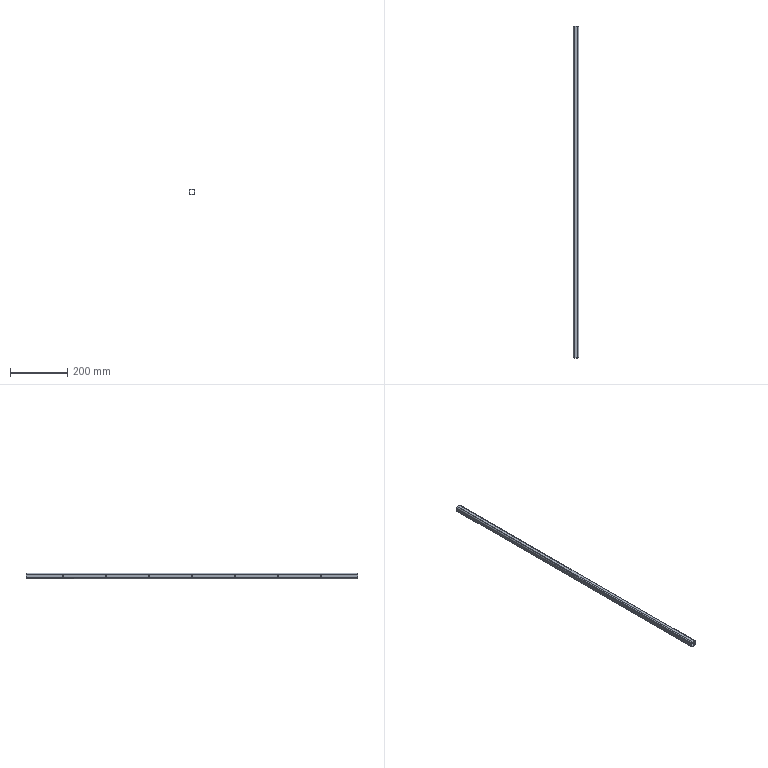Part | NX | features BREP 1 | 1 solid | 52 faces | box 20 x 1158 x 20 mm | volume 150717 mm3 | cylinder 28 | plane 24 | commonest cylinder face diameters 4 x16 6 x8 10 x4